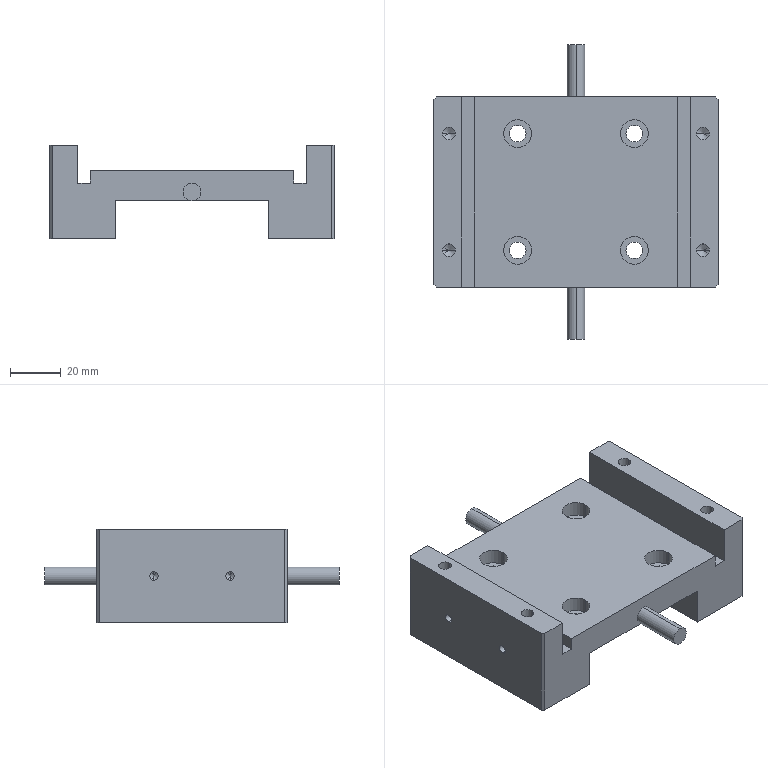Part | NX | features BREP 1 | 1 solid | 72 faces | box 112 x 116 x 37 mm | volume 169084 mm3 | cylinder 32 | plane 28 | cone 12 | commonest cylinder face diameters 5 x8 6.6 x8 11 x8 3.3 x4 7 x4